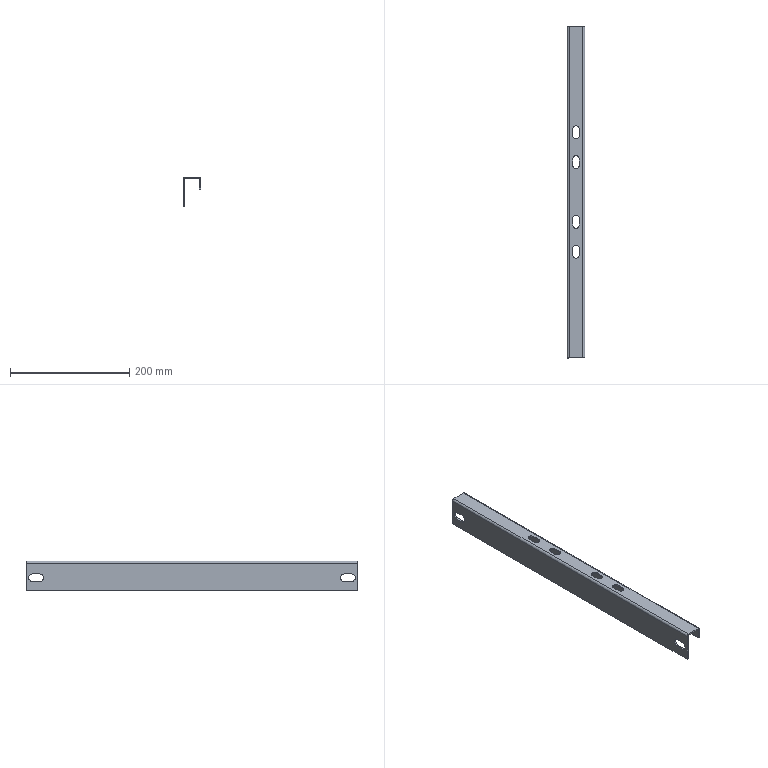Part | SolidWorks | features ICE 2, FlatPattern 1, SMBaseFlange 1, SheetMetal 1 | 1 solid | 46 faces | box 30 x 557 x 50 mm | volume 125994 mm3 | plane 30 | cylinder 16 | commonest cylinder face diameters 11 x8 13 x4 2 x2 7 x2
STEP:
#1=CARTESIAN_POINT('',(0.,278.5,-3.5));
#2=VERTEX_POINT('',#1);
#3=CARTESIAN_POINT('',(2.5,278.5,-3.5));
#4=VERTEX_POINT('',#3);
#5=CARTESIAN_POINT('',(0.,278.5,-3.5));
#6=DIRECTION('',(1.,0.,0.));
#7=VECTOR('',#6,1000.);
#8=LINE('',#5,#7);
#9=EDGE_CURVE('',#2,#4,#8,.T.);
#10=ORIENTED_EDGE('',*,*,#9,.F.);
#11=CARTESIAN_POINT('',(3.5,278.5,0.));
#12=VERTEX_POINT('',#11);
#13=CARTESIAN_POINT('',(3.5,278.5,-3.5));
#14=DIRECTION('',(0.,1.,0.));
#15=DIRECTION('',(0.,0.,-1.));
#16=AXIS2_PLACEMENT_3D('',#13,#14,#15);
#17=CIRCLE('',#16,3.5);
#18=EDGE_CURVE('',#2,#12,#17,.T.);
#19=ORIENTED_EDGE('',*,*,#18,.T.);
#20=CARTESIAN_POINT('',(3.5,278.5,-2.5));
#21=VERTEX_POINT('',#20);
#22=CARTESIAN_POINT('',(3.5,278.5,-2.5));
#23=DIRECTION('',(0.,0.,1.));
#24=VECTOR('',#23,1000.);
#25=LINE('',#22,#24);
#26=EDGE_CURVE('',#21,#12,#25,.T.);
#27=ORIENTED_EDGE('',*,*,#26,.F.);
#28=CARTESIAN_POINT('',(3.5,278.5,-3.5));
#29=DIRECTION('',(0.,1.,0.));
#30=DIRECTION('',(1.,0.,0.));
#31=AXIS2_PLACEMENT_3D('',#28,#29,#30);
#32=CIRCLE('',#31,1.);
#33=EDGE_CURVE('',#4,#21,#32,.T.);
#34=ORIENTED_EDGE('',*,*,#33,.F.);
#35=EDGE_LOOP('',(#10,#19,#27,#34));
#36=FACE_OUTER_BOUND('',#35,.T.);
#37=CARTESIAN_POINT('',(0.,278.5,-3.5));
#38=DIRECTION('',(0.,1.,0.));
#39=DIRECTION('',(0.,0.,1.));
#40=AXIS2_PLACEMENT_3D('',#37,#38,#39);
#41=PLANE('',#40);
#42=ADVANCED_FACE('',(#36),#41,.T.);
#43=CARTESIAN_POINT('',(0.,278.5,-50.));
#44=VERTEX_POINT('',#43);
#45=CARTESIAN_POINT('',(0.,278.5,0.));
#46=DIRECTION('',(0.,0.,1.));
#47=VECTOR('',#46,1000.);
#48=LINE('',#45,#47);
#49=EDGE_CURVE('',#44,#2,#48,.T.);
#50=ORIENTED_EDGE('',*,*,#49,.T.);
#51=ORIENTED_EDGE('',*,*,#9,.T.);
#52=CARTESIAN_POINT('',(2.5,278.5,-50.));
#53=VERTEX_POINT('',#52);
#54=CARTESIAN_POINT('',(2.5,278.5,0.));
#55=DIRECTION('',(0.,0.,1.));
#56=VECTOR('',#55,1000.);
#57=LINE('',#54,#56);
#58=EDGE_CURVE('',#53,#4,#57,.T.);
#59=ORIENTED_EDGE('',*,*,#58,.F.);
#60=CARTESIAN_POINT('',(0.,278.5,-50.));
#61=DIRECTION('',(1.,0.,0.));
#62=VECTOR('',#61,1000.);
#63=LINE('',#60,#62);
#64=EDGE_CURVE('',#44,#53,#63,.T.);
#65=ORIENTED_EDGE('',*,*,#64,.F.);
#66=EDGE_LOOP('',(#50,#51,#59,#65));
#67=FACE_OUTER_BOUND('',#66,.T.);
#68=CARTESIAN_POINT('',(3.5,278.5,-2.5));
#69=DIRECTION('',(0.,1.,0.));
#70=DIRECTION('',(0.,0.,1.));
#71=AXIS2_PLACEMENT_3D('',#68,#69,#70);
#72=PLANE('',#71);
#73=ADVANCED_FACE('',(#67),#72,.T.);
#74=CARTESIAN_POINT('',(3.5,-278.5,0.));
#75=VERTEX_POINT('',#74);
#76=CARTESIAN_POINT('',(3.5,-278.5,-2.5));
#77=VERTEX_POINT('',#76);
#78=CARTESIAN_POINT('',(3.5,-278.5,0.));
#79=DIRECTION('',(0.,0.,-1.));
#80=VECTOR('',#79,1000.);
#81=LINE('',#78,#80);
#82=EDGE_CURVE('',#75,#77,#81,.T.);
#83=ORIENTED_EDGE('',*,*,#82,.F.);
#84=CARTESIAN_POINT('',(0.,-278.5,-3.5));
#85=VERTEX_POINT('',#84);
#86=CARTESIAN_POINT('',(3.5,-278.5,-3.5));
#87=DIRECTION('',(0.,1.,0.));
#88=DIRECTION('',(0.,0.,-1.));
#89=AXIS2_PLACEMENT_3D('',#86,#87,#88);
#90=CIRCLE('',#89,3.5);
#91=EDGE_CURVE('',#85,#75,#90,.T.);
#92=ORIENTED_EDGE('',*,*,#91,.F.);
#93=CARTESIAN_POINT('',(2.5,-278.5,-3.5));
#94=VERTEX_POINT('',#93);
#95=CARTESIAN_POINT('',(2.5,-278.5,-3.5));
#96=DIRECTION('',(-1.,0.,0.));
#97=VECTOR('',#96,1000.);
#98=LINE('',#95,#97);
#99=EDGE_CURVE('',#94,#85,#98,.T.);
#100=ORIENTED_EDGE('',*,*,#99,.F.);
#101=CARTESIAN_POINT('',(3.5,-278.5,-3.5));
#102=DIRECTION('',(0.,1.,0.));
#103=DIRECTION('',(1.,0.,0.));
#104=AXIS2_PLACEMENT_3D('',#101,#102,#103);
#105=CIRCLE('',#104,1.);
#106=EDGE_CURVE('',#94,#77,#105,.T.);
#107=ORIENTED_EDGE('',*,*,#106,.T.);
#108=EDGE_LOOP('',(#83,#92,#100,#107));
#109=FACE_OUTER_BOUND('',#108,.T.);
#110=CARTESIAN_POINT('',(3.5,-278.5,0.));
#111=DIRECTION('',(0.,-1.,0.));
#112=DIRECTION('',(0.,0.,-1.));
#113=AXIS2_PLACEMENT_3D('',#110,#111,#112);
#114=PLANE('',#113);
#115=ADVANCED_FACE('',(#109),#114,.T.);
#116=CARTESIAN_POINT('',(26.5,-278.5,0.));
#117=VERTEX_POINT('',#116);
#118=CARTESIAN_POINT('',(0.,-278.5,0.));
#119=DIRECTION('',(1.,0.,0.));
#120=VECTOR('',#119,1000.);
#121=LINE('',#118,#120);
#122=EDGE_CURVE('',#75,#117,#121,.T.);
#123=ORIENTED_EDGE('',*,*,#122,.F.);
#124=ORIENTED_EDGE('',*,*,#82,.T.);
#125=CARTESIAN_POINT('',(26.5,-278.5,-2.5));
#126=VERTEX_POINT('',#125);
#127=CARTESIAN_POINT('',(0.,-278.5,-2.5));
#128=DIRECTION('',(1.,0.,0.));
#129=VECTOR('',#128,1000.);
#130=LINE('',#127,#129);
#131=EDGE_CURVE('',#77,#126,#130,.T.);
#132=ORIENTED_EDGE('',*,*,#131,.T.);
#133=CARTESIAN_POINT('',(26.5,-278.5,-2.5));
#134=DIRECTION('',(0.,0.,1.));
#135=VECTOR('',#134,1000.);
#136=LINE('',#133,#135);
#137=EDGE_CURVE('',#126,#117,#136,.T.);
#138=ORIENTED_EDGE('',*,*,#137,.T.);
#139=EDGE_LOOP('',(#123,#124,#132,#138));
#140=FACE_OUTER_BOUND('',#139,.T.);
#141=CARTESIAN_POINT('',(2.5,-278.5,-3.5));
#142=DIRECTION('',(0.,-1.,0.));
#143=DIRECTION('',(0.,0.,-1.));
#144=AXIS2_PLACEMENT_3D('',#141,#142,#143);
#145=PLANE('',#144);
#146=ADVANCED_FACE('',(#140),#145,.T.);
#147=CARTESIAN_POINT('',(26.5,278.5,0.));
#148=VERTEX_POINT('',#147);
#149=CARTESIAN_POINT('',(26.5,278.5,-2.5));
#150=VERTEX_POINT('',#149);
#151=CARTESIAN_POINT('',(26.5,278.5,0.));
#152=DIRECTION('',(0.,0.,-1.));
#153=VECTOR('',#152,1000.);
#154=LINE('',#151,#153);
#155=EDGE_CURVE('',#148,#150,#154,.T.);
#156=ORIENTED_EDGE('',*,*,#155,.F.);
#157=CARTESIAN_POINT('',(30.,278.5,-3.5));
#158=VERTEX_POINT('',#157);
#159=CARTESIAN_POINT('',(26.5,278.5,-3.5));
#160=DIRECTION('',(0.,1.,0.));
#161=DIRECTION('',(0.,0.,-1.));
#162=AXIS2_PLACEMENT_3D('',#159,#160,#161);
#163=CIRCLE('',#162,3.5);
#164=EDGE_CURVE('',#148,#158,#163,.T.);
#165=ORIENTED_EDGE('',*,*,#164,.T.);
#166=CARTESIAN_POINT('',(27.5,278.5,-3.5));
#167=VERTEX_POINT('',#166);
#168=CARTESIAN_POINT('',(27.5,278.5,-3.5));
#169=DIRECTION('',(1.,0.,0.));
#170=VECTOR('',#169,1000.);
#171=LINE('',#168,#170);
#172=EDGE_CURVE('',#167,#158,#171,.T.);
#173=ORIENTED_EDGE('',*,*,#172,.F.);
#174=CARTESIAN_POINT('',(26.5,278.5,-3.5));
#175=DIRECTION('',(0.,1.,0.));
#176=DIRECTION('',(1.,0.,0.));
#177=AXIS2_PLACEMENT_3D('',#174,#175,#176);
#178=CIRCLE('',#177,1.);
#179=EDGE_CURVE('',#150,#167,#178,.T.);
#180=ORIENTED_EDGE('',*,*,#179,.F.);
#181=EDGE_LOOP('',(#156,#165,#173,#180));
#182=FACE_OUTER_BOUND('',#181,.T.);
#183=CARTESIAN_POINT('',(26.5,278.5,0.));
#184=DIRECTION('',(0.,1.,0.));
#185=DIRECTION('',(0.,0.,1.));
#186=AXIS2_PLACEMENT_3D('',#183,#184,#185);
#187=PLANE('',#186);
#188=ADVANCED_FACE('',(#182),#187,.T.);
#189=CARTESIAN_POINT('',(0.,278.5,0.));
#190=DIRECTION('',(1.,0.,0.));
#191=VECTOR('',#190,1000.);
#192=LINE('',#189,#191);
#193=EDGE_CURVE('',#12,#148,#192,.T.);
#194=ORIENTED_EDGE('',*,*,#193,.T.);
#195=ORIENTED_EDGE('',*,*,#155,.T.);
#196=CARTESIAN_POINT('',(0.,278.5,-2.5));
#197=DIRECTION('',(1.,0.,0.));
#198=VECTOR('',#197,1000.);
#199=LINE('',#196,#198);
#200=EDGE_CURVE('',#21,#150,#199,.T.);
#201=ORIENTED_EDGE('',*,*,#200,.F.);
#202=ORIENTED_EDGE('',*,*,#26,.T.);
#203=EDGE_LOOP('',(#194,#195,#201,#202));
#204=FACE_OUTER_BOUND('',#203,.T.);
#205=CARTESIAN_POINT('',(27.5,278.5,-3.5));
#206=DIRECTION('',(0.,1.,0.));
#207=DIRECTION('',(0.,0.,1.));
#208=AXIS2_PLACEMENT_3D('',#205,#206,#207);
#209=PLANE('',#208);
#210=ADVANCED_FACE('',(#204),#209,.T.);
#211=CARTESIAN_POINT('',(30.,-278.5,-3.5));
#212=VERTEX_POINT('',#211);
#213=CARTESIAN_POINT('',(27.5,-278.5,-3.5));
#214=VERTEX_POINT('',#213);
#215=CARTESIAN_POINT('',(30.,-278.5,-3.5));
#216=DIRECTION('',(-1.,0.,0.));
#217=VECTOR('',#216,1000.);
#218=LINE('',#215,#217);
#219=EDGE_CURVE('',#212,#214,#218,.T.);
#220=ORIENTED_EDGE('',*,*,#219,.F.);
#221=CARTESIAN_POINT('',(26.5,-278.5,-3.5));
#222=DIRECTION('',(0.,1.,0.));
#223=DIRECTION('',(0.,0.,-1.));
#224=AXIS2_PLACEMENT_3D('',#221,#222,#223);
#225=CIRCLE('',#224,3.5);
#226=EDGE_CURVE('',#117,#212,#225,.T.);
#227=ORIENTED_EDGE('',*,*,#226,.F.);
#228=ORIENTED_EDGE('',*,*,#137,.F.);
#229=CARTESIAN_POINT('',(26.5,-278.5,-3.5));
#230=DIRECTION('',(0.,1.,0.));
#231=DIRECTION('',(1.,0.,0.));
#232=AXIS2_PLACEMENT_3D('',#229,#230,#231);
#233=CIRCLE('',#232,1.);
#234=EDGE_CURVE('',#126,#214,#233,.T.);
#235=ORIENTED_EDGE('',*,*,#234,.T.);
#236=EDGE_LOOP('',(#220,#227,#228,#235));
#237=FACE_OUTER_BOUND('',#236,.T.);
#238=CARTESIAN_POINT('',(30.,-278.5,-3.5));
#239=DIRECTION('',(0.,-1.,0.));
#240=DIRECTION('',(0.,0.,-1.));
#241=AXIS2_PLACEMENT_3D('',#238,#239,#240);
#242=PLANE('',#241);
#243=ADVANCED_FACE('',(#237),#242,.T.);
#244=CARTESIAN_POINT('',(30.,-278.5,-20.));
#245=VERTEX_POINT('',#244);
#246=CARTESIAN_POINT('',(30.,-278.5,0.));
#247=DIRECTION('',(0.,0.,-1.));
#248=VECTOR('',#247,1000.);
#249=LINE('',#246,#248);
#250=EDGE_CURVE('',#212,#245,#249,.T.);
#251=ORIENTED_EDGE('',*,*,#250,.F.);
#252=ORIENTED_EDGE('',*,*,#219,.T.);
#253=CARTESIAN_POINT('',(27.5,-278.5,-20.));
#254=VERTEX_POINT('',#253);
#255=CARTESIAN_POINT('',(27.5,-278.5,0.));
#256=DIRECTION('',(0.,0.,-1.));
#257=VECTOR('',#256,1000.);
#258=LINE('',#255,#257);
#259=EDGE_CURVE('',#214,#254,#258,.T.);
#260=ORIENTED_EDGE('',*,*,#259,.T.);
#261=CARTESIAN_POINT('',(27.5,-278.5,-20.));
#262=DIRECTION('',(1.,0.,0.));
#263=VECTOR('',#262,1000.);
#264=LINE('',#261,#263);
#265=EDGE_CURVE('',#254,#245,#264,.T.);
#266=ORIENTED_EDGE('',*,*,#265,.T.);
#267=EDGE_LOOP('',(#251,#252,#260,#266));
#268=FACE_OUTER_BOUND('',#267,.T.);
#269=CARTESIAN_POINT('',(26.5,-278.5,-2.5));
#270=DIRECTION('',(0.,-1.,0.));
#271=DIRECTION('',(0.,0.,-1.));
#272=AXIS2_PLACEMENT_3D('',#269,#270,#271);
#273=PLANE('',#272);
#274=ADVANCED_FACE('',(#268),#273,.T.);
#275=ORIENTED_EDGE('',*,*,#250,.T.);
#276=CARTESIAN_POINT('',(30.,278.5,-20.));
#277=VERTEX_POINT('',#276);
#278=CARTESIAN_POINT('',(30.,278.5,-20.));
#279=DIRECTION('',(0.,-1.,0.));
#280=VECTOR('',#279,1000.);
#281=LINE('',#278,#280);
#282=EDGE_CURVE('',#277,#245,#281,.T.);
#283=ORIENTED_EDGE('',*,*,#282,.F.);
#284=CARTESIAN_POINT('',(30.,278.5,0.));
#285=DIRECTION('',(0.,0.,-1.));
#286=VECTOR('',#285,1000.);
#287=LINE('',#284,#286);
#288=EDGE_CURVE('',#158,#277,#287,.T.);
#289=ORIENTED_EDGE('',*,*,#288,.F.);
#290=CARTESIAN_POINT('',(30.,278.5,-3.5));
#291=DIRECTION('',(0.,-1.,0.));
#292=VECTOR('',#291,1000.);
#293=LINE('',#290,#292);
#294=EDGE_CURVE('',#158,#212,#293,.T.);
#295=ORIENTED_EDGE('',*,*,#294,.T.);
#296=EDGE_LOOP('',(#275,#283,#289,#295));
#297=FACE_OUTER_BOUND('',#296,.T.);
#298=CARTESIAN_POINT('',(30.,278.5,0.));
#299=DIRECTION('',(-1.,0.,0.));
#300=DIRECTION('',(0.,0.,1.));
#301=AXIS2_PLACEMENT_3D('',#298,#299,#300);
#302=PLANE('',#301);
#303=ADVANCED_FACE('',(#297),#302,.F.);
#304=ORIENTED_EDGE('',*,*,#265,.F.);
#305=CARTESIAN_POINT('',(27.5,278.5,-20.));
#306=VERTEX_POINT('',#305);
#307=CARTESIAN_POINT('',(27.5,278.5,-20.));
#308=DIRECTION('',(0.,-1.,0.));
#309=VECTOR('',#308,1000.);
#310=LINE('',#307,#309);
#311=EDGE_CURVE('',#306,#254,#310,.T.);
#312=ORIENTED_EDGE('',*,*,#311,.F.);
#313=CARTESIAN_POINT('',(27.5,278.5,-20.));
#314=DIRECTION('',(1.,0.,0.));
#315=VECTOR('',#314,1000.);
#316=LINE('',#313,#315);
#317=EDGE_CURVE('',#306,#277,#316,.T.);
#318=ORIENTED_EDGE('',*,*,#317,.T.);
#319=ORIENTED_EDGE('',*,*,#282,.T.);
#320=EDGE_LOOP('',(#304,#312,#318,#319));
#321=FACE_OUTER_BOUND('',#320,.T.);
#322=CARTESIAN_POINT('',(27.5,278.5,-20.));
#323=DIRECTION('',(0.,0.,-1.));
#324=DIRECTION('',(-1.,0.,0.));
#325=AXIS2_PLACEMENT_3D('',#322,#323,#324);
#326=PLANE('',#325);
#327=ADVANCED_FACE('',(#321),#326,.T.);
#328=ORIENTED_EDGE('',*,*,#259,.F.);
#329=CARTESIAN_POINT('',(27.5,278.5,-3.5));
#330=DIRECTION('',(0.,-1.,0.));
#331=VECTOR('',#330,1000.);
#332=LINE('',#329,#331);
#333=EDGE_CURVE('',#167,#214,#332,.T.);
#334=ORIENTED_EDGE('',*,*,#333,.F.);
#335=CARTESIAN_POINT('',(27.5,278.5,0.));
#336=DIRECTION('',(0.,0.,-1.));
#337=VECTOR('',#336,1000.);
#338=LINE('',#335,#337);
#339=EDGE_CURVE('',#167,#306,#338,.T.);
#340=ORIENTED_EDGE('',*,*,#339,.T.);
#341=ORIENTED_EDGE('',*,*,#311,.T.);
#342=EDGE_LOOP('',(#328,#334,#340,#341));
#343=FACE_OUTER_BOUND('',#342,.T.);
#344=CARTESIAN_POINT('',(27.5,278.5,0.));
#345=DIRECTION('',(-1.,0.,0.));
#346=DIRECTION('',(0.,0.,1.));
#347=AXIS2_PLACEMENT_3D('',#344,#345,#346);
#348=PLANE('',#347);
#349=ADVANCED_FACE('',(#343),#348,.T.);
#350=ORIENTED_EDGE('',*,*,#234,.F.);
#351=CARTESIAN_POINT('',(26.5,278.5,-2.5));
#352=DIRECTION('',(0.,-1.,0.));
#353=VECTOR('',#352,1000.);
#354=LINE('',#351,#353);
#355=EDGE_CURVE('',#150,#126,#354,.T.);
#356=ORIENTED_EDGE('',*,*,#355,.F.);
#357=ORIENTED_EDGE('',*,*,#179,.T.);
#358=ORIENTED_EDGE('',*,*,#333,.T.);
#359=EDGE_LOOP('',(#350,#356,#357,#358));
#360=FACE_OUTER_BOUND('',#359,.T.);
#361=CARTESIAN_POINT('',(26.5,278.5,-3.5));
#362=DIRECTION('',(0.,-1.,0.));
#363=DIRECTION('',(0.,0.,-1.));
#364=AXIS2_PLACEMENT_3D('',#361,#362,#363);
#365=CYLINDRICAL_SURFACE('',#364,1.);
#366=ADVANCED_FACE('',(#360),#365,.F.);
#367=CARTESIAN_POINT('',(20.5,-105.5,-2.5));
#368=VERTEX_POINT('',#367);
#369=CARTESIAN_POINT('',(9.5,-105.5,-2.5));
#370=VERTEX_POINT('',#369);
#371=CARTESIAN_POINT('',(15.,-105.5,-2.5));
#372=DIRECTION('',(0.,0.,-1.));
#373=DIRECTION('',(-1.,0.,0.));
#374=AXIS2_PLACEMENT_3D('',#371,#372,#373);
#375=CIRCLE('',#374,5.5);
#376=EDGE_CURVE('',#368,#370,#375,.T.);
#377=ORIENTED_EDGE('',*,*,#376,.F.);
#378=CARTESIAN_POINT('',(20.5,-94.5,-2.5));
#379=VERTEX_POINT('',#378);
#380=CARTESIAN_POINT('',(20.5,-105.5,-2.5));
#381=DIRECTION('',(0.,-1.,0.));
#382=VECTOR('',#381,1000.);
#383=LINE('',#380,#382);
#384=EDGE_CURVE('',#379,#368,#383,.T.);
#385=ORIENTED_EDGE('',*,*,#384,.F.);
#386=CARTESIAN_POINT('',(9.5,-94.5,-2.5));
#387=VERTEX_POINT('',#386);
#388=CARTESIAN_POINT('',(15.,-94.5,-2.5));
#389=DIRECTION('',(0.,0.,-1.));
#390=DIRECTION('',(-1.,0.,0.));
#391=AXIS2_PLACEMENT_3D('',#388,#389,#390);
#392=CIRCLE('',#391,5.5);
#393=EDGE_CURVE('',#387,#379,#392,.T.);
#394=ORIENTED_EDGE('',*,*,#393,.F.);
#395=CARTESIAN_POINT('',(9.5,-105.5,-2.5));
#396=DIRECTION('',(0.,1.,0.));
#397=VECTOR('',#396,1000.);
#398=LINE('',#395,#397);
#399=EDGE_CURVE('',#370,#387,#398,.T.);
#400=ORIENTED_EDGE('',*,*,#399,.F.);
#401=EDGE_LOOP('',(#377,#385,#394,#400));
#402=FACE_BOUND('',#401,.T.);
#403=CARTESIAN_POINT('',(9.5,105.5,-2.5));
#404=VERTEX_POINT('',#403);
#405=CARTESIAN_POINT('',(20.5,105.5,-2.5));
#406=VERTEX_POINT('',#405);
#407=CARTESIAN_POINT('',(15.,105.5,-2.5));
#408=DIRECTION('',(0.,0.,-1.));
#409=DIRECTION('',(1.,0.,0.));
#410=AXIS2_PLACEMENT_3D('',#407,#408,#409);
#411=CIRCLE('',#410,5.5);
#412=EDGE_CURVE('',#404,#406,#411,.T.);
#413=ORIENTED_EDGE('',*,*,#412,.F.);
#414=CARTESIAN_POINT('',(9.5,94.5,-2.5));
#415=VERTEX_POINT('',#414);
#416=CARTESIAN_POINT('',(9.5,105.5,-2.5));
#417=DIRECTION('',(0.,1.,0.));
#418=VECTOR('',#417,1000.);
#419=LINE('',#416,#418);
#420=EDGE_CURVE('',#415,#404,#419,.T.);
#421=ORIENTED_EDGE('',*,*,#420,.F.);
#422=CARTESIAN_POINT('',(20.5,94.5,-2.5));
#423=VERTEX_POINT('',#422);
#424=CARTESIAN_POINT('',(15.,94.5,-2.5));
#425=DIRECTION('',(0.,0.,-1.));
#426=DIRECTION('',(1.,0.,0.));
#427=AXIS2_PLACEMENT_3D('',#424,#425,#426);
#428=CIRCLE('',#427,5.5);
#429=EDGE_CURVE('',#423,#415,#428,.T.);
#430=ORIENTED_EDGE('',*,*,#429,.F.);
#431=CARTESIAN_POINT('',(20.5,105.5,-2.5));
#432=DIRECTION('',(0.,-1.,0.));
#433=VECTOR('',#432,1000.);
#434=LINE('',#431,#433);
#435=EDGE_CURVE('',#406,#423,#434,.T.);
#436=ORIENTED_EDGE('',*,*,#435,.F.);
#437=EDGE_LOOP('',(#413,#421,#430,#436));
#438=FACE_BOUND('',#437,.T.);
#439=CARTESIAN_POINT('',(9.5,55.5,-2.5));
#440=VERTEX_POINT('',#439);
#441=CARTESIAN_POINT('',(20.5,55.5,-2.5));
#442=VERTEX_POINT('',#441);
#443=CARTESIAN_POINT('',(15.,55.5,-2.5));
#444=DIRECTION('',(0.,0.,-1.));
#445=DIRECTION('',(1.,0.,0.));
#446=AXIS2_PLACEMENT_3D('',#443,#444,#445);
#447=CIRCLE('',#446,5.5);
#448=EDGE_CURVE('',#440,#442,#447,.T.);
#449=ORIENTED_EDGE('',*,*,#448,.F.);
#450=CARTESIAN_POINT('',(9.5,44.5,-2.5));
#451=VERTEX_POINT('',#450);
#452=CARTESIAN_POINT('',(9.5,55.5,-2.5));
#453=DIRECTION('',(0.,1.,0.));
#454=VECTOR('',#453,1000.);
#455=LINE('',#452,#454);
#456=EDGE_CURVE('',#451,#440,#455,.T.);
#457=ORIENTED_EDGE('',*,*,#456,.F.);
#458=CARTESIAN_POINT('',(20.5,44.5,-2.5));
#459=VERTEX_POINT('',#458);
#460=CARTESIAN_POINT('',(15.,44.5,-2.5));
#461=DIRECTION('',(0.,0.,-1.));
#462=DIRECTION('',(1.,0.,0.));
#463=AXIS2_PLACEMENT_3D('',#460,#461,#462);
#464=CIRCLE('',#463,5.5);
#465=EDGE_CURVE('',#459,#451,#464,.T.);
#466=ORIENTED_EDGE('',*,*,#465,.F.);
#467=CARTESIAN_POINT('',(20.5,55.5,-2.5));
#468=DIRECTION('',(0.,-1.,0.));
#469=VECTOR('',#468,1000.);
#470=LINE('',#467,#469);
#471=EDGE_CURVE('',#442,#459,#470,.T.);
#472=ORIENTED_EDGE('',*,*,#471,.F.);
#473=EDGE_LOOP('',(#449,#457,#466,#472));
#474=FACE_BOUND('',#473,.T.);
#475=CARTESIAN_POINT('',(20.5,-55.5,-2.5));
#476=VERTEX_POINT('',#475);
#477=CARTESIAN_POINT('',(9.5,-55.5,-2.5));
#478=VERTEX_POINT('',#477);
#479=CARTESIAN_POINT('',(15.,-55.5,-2.5));
#480=DIRECTION('',(0.,0.,-1.));
#481=DIRECTION('',(-1.,0.,0.));
#482=AXIS2_PLACEMENT_3D('',#479,#480,#481);
#483=CIRCLE('',#482,5.5);
#484=EDGE_CURVE('',#476,#478,#483,.T.);
#485=ORIENTED_EDGE('',*,*,#484,.F.);
#486=CARTESIAN_POINT('',(20.5,-44.5,-2.5));
#487=VERTEX_POINT('',#486);
#488=CARTESIAN_POINT('',(20.5,-55.5,-2.5));
#489=DIRECTION('',(0.,-1.,0.));
#490=VECTOR('',#489,1000.);
#491=LINE('',#488,#490);
#492=EDGE_CURVE('',#487,#476,#491,.T.);
#493=ORIENTED_EDGE('',*,*,#492,.F.);
#494=CARTESIAN_POINT('',(9.5,-44.5,-2.5));
#495=VERTEX_POINT('',#494);
#496=CARTESIAN_POINT('',(15.,-44.5,-2.5));
#497=DIRECTION('',(0.,0.,-1.));
#498=DIRECTION('',(-1.,0.,0.));
#499=AXIS2_PLACEMENT_3D('',#496,#497,#498);
#500=CIRCLE('',#499,5.5);
#501=EDGE_CURVE('',#495,#487,#500,.T.);
#502=ORIENTED_EDGE('',*,*,#501,.F.);
#503=CARTESIAN_POINT('',(9.5,-55.5,-2.5));
#504=DIRECTION('',(0.,1.,0.));
#505=VECTOR('',#504,1000.);
#506=LINE('',#503,#505);
#507=EDGE_CURVE('',#478,#495,#506,.T.);
#508=ORIENTED_EDGE('',*,*,#507,.F.);
#509=EDGE_LOOP('',(#485,#493,#502,#508));
#510=FACE_BOUND('',#509,.T.);
#511=ORIENTED_EDGE('',*,*,#131,.F.);
#512=CARTESIAN_POINT('',(3.5,278.5,-2.5));
#513=DIRECTION('',(0.,-1.,0.));
#514=VECTOR('',#513,1000.);
#515=LINE('',#512,#514);
#516=EDGE_CURVE('',#21,#77,#515,.T.);
#517=ORIENTED_EDGE('',*,*,#516,.F.);
#518=ORIENTED_EDGE('',*,*,#200,.T.);
#519=ORIENTED_EDGE('',*,*,#355,.T.);
#520=EDGE_LOOP('',(#511,#517,#518,#519));
#521=FACE_OUTER_BOUND('',#520,.T.);
#522=CARTESIAN_POINT('',(0.,278.5,-2.5));
#523=DIRECTION('',(0.,0.,-1.));
#524=DIRECTION('',(-1.,0.,0.));
#525=AXIS2_PLACEMENT_3D('',#522,#523,#524);
#526=PLANE('',#525);
#527=ADVANCED_FACE('',(#402,#438,#474,#510,#521),#526,.T.);
#528=ORIENTED_EDGE('',*,*,#106,.F.);
#529=CARTESIAN_POINT('',(2.5,278.5,-3.5));
#530=DIRECTION('',(0.,-1.,0.));
#531=VECTOR('',#530,1000.);
#532=LINE('',#529,#531);
#533=EDGE_CURVE('',#4,#94,#532,.T.);
#534=ORIENTED_EDGE('',*,*,#533,.F.);
#535=ORIENTED_EDGE('',*,*,#33,.T.);
#536=ORIENTED_EDGE('',*,*,#516,.T.);
#537=EDGE_LOOP('',(#528,#534,#535,#536));
#538=FACE_OUTER_BOUND('',#537,.T.);
#539=CARTESIAN_POINT('',(3.5,278.5,-3.5));
#540=DIRECTION('',(0.,-1.,0.));
#541=DIRECTION('',(0.,0.,-1.));
#542=AXIS2_PLACEMENT_3D('',#539,#540,#541);
#543=CYLINDRICAL_SURFACE('',#542,1.);
#544=ADVANCED_FACE('',(#538),#543,.F.);
#545=CARTESIAN_POINT('',(2.5,-267.5,-21.5));
#546=VERTEX_POINT('',#545);
#547=CARTESIAN_POINT('',(2.5,-267.5,-34.5));
#548=VERTEX_POINT('',#547);
#549=CARTESIAN_POINT('',(2.5,-267.5,-28.));
#550=DIRECTION('',(1.,0.,0.));
#551=DIRECTION('',(0.,0.,-1.));
#552=AXIS2_PLACEMENT_3D('',#549,#550,#551);
#553=CIRCLE('',#552,6.5);
#554=EDGE_CURVE('',#546,#548,#553,.T.);
#555=ORIENTED_EDGE('',*,*,#554,.F.);
#556=CARTESIAN_POINT('',(2.5,-255.5,-21.5));
#557=VERTEX_POINT('',#556);
#558=CARTESIAN_POINT('',(2.5,278.5,-21.5));
#559=DIRECTION('',(0.,-1.,0.));
#560=VECTOR('',#559,1000.);
#561=LINE('',#558,#560);
#562=EDGE_CURVE('',#557,#546,#561,.T.);
#563=ORIENTED_EDGE('',*,*,#562,.F.);
#564=CARTESIAN_POINT('',(2.5,-255.5,-34.5));
#565=VERTEX_POINT('',#564);
#566=CARTESIAN_POINT('',(2.5,-255.5,-28.));
#567=DIRECTION('',(1.,0.,0.));
#568=DIRECTION('',(0.,0.,-1.));
#569=AXIS2_PLACEMENT_3D('',#566,#567,#568);
#570=CIRCLE('',#569,6.5);
#571=EDGE_CURVE('',#565,#557,#570,.T.);
#572=ORIENTED_EDGE('',*,*,#571,.F.);
#573=CARTESIAN_POINT('',(2.5,278.5,-34.5));
#574=DIRECTION('',(0.,1.,0.));
#575=VECTOR('',#574,1000.);
#576=LINE('',#573,#575);
#577=EDGE_CURVE('',#548,#565,#576,.T.);
#578=ORIENTED_EDGE('',*,*,#577,.F.);
#579=EDGE_LOOP('',(#555,#563,#572,#578));
#580=FACE_BOUND('',#579,.T.);
#581=CARTESIAN_POINT('',(2.5,267.5,-34.5));
#582=VERTEX_POINT('',#581);
#583=CARTESIAN_POINT('',(2.5,267.5,-21.5));
#584=VERTEX_POINT('',#583);
#585=CARTESIAN_POINT('',(2.5,267.5,-28.));
#586=DIRECTION('',(1.,0.,0.));
#587=DIRECTION('',(0.,0.,-1.));
#588=AXIS2_PLACEMENT_3D('',#585,#586,#587);
#589=CIRCLE('',#588,6.5);
#590=EDGE_CURVE('',#582,#584,#589,.T.);
#591=ORIENTED_EDGE('',*,*,#590,.F.);
#592=CARTESIAN_POINT('',(2.5,255.5,-34.5));
#593=VERTEX_POINT('',#592);
#594=CARTESIAN_POINT('',(2.5,278.5,-34.5));
#595=DIRECTION('',(0.,1.,0.));
#596=VECTOR('',#595,1000.);
#597=LINE('',#594,#596);
#598=EDGE_CURVE('',#593,#582,#597,.T.);
#599=ORIENTED_EDGE('',*,*,#598,.F.);
#600=CARTESIAN_POINT('',(2.5,255.5,-21.5));
#601=VERTEX_POINT('',#600);
#602=CARTESIAN_POINT('',(2.5,255.5,-28.));
#603=DIRECTION('',(1.,0.,0.));
#604=DIRECTION('',(0.,0.,-1.));
#605=AXIS2_PLACEMENT_3D('',#602,#603,#604);
#606=CIRCLE('',#605,6.5);
#607=EDGE_CURVE('',#601,#593,#606,.T.);
#608=ORIENTED_EDGE('',*,*,#607,.F.);
#609=CARTESIAN_POINT('',(2.5,278.5,-21.5));
#610=DIRECTION('',(0.,-1.,0.));
#611=VECTOR('',#610,1000.);
#612=LINE('',#609,#611);
#613=EDGE_CURVE('',#584,#601,#612,.T.);
#614=ORIENTED_EDGE('',*,*,#613,.F.);
#615=EDGE_LOOP('',(#591,#599,#608,#614));
#616=FACE_BOUND('',#615,.T.);
#617=CARTESIAN_POINT('',(2.5,-278.5,-50.));
#618=VERTEX_POINT('',#617);
#619=CARTESIAN_POINT('',(2.5,-278.5,0.));
#620=DIRECTION('',(0.,0.,1.));
#621=VECTOR('',#620,1000.);
#622=LINE('',#619,#621);
#623=EDGE_CURVE('',#618,#94,#622,.T.);
#624=ORIENTED_EDGE('',*,*,#623,.F.);
#625=CARTESIAN_POINT('',(2.5,278.5,-50.));
#626=DIRECTION('',(0.,-1.,0.));
#627=VECTOR('',#626,1000.);
#628=LINE('',#625,#627);
#629=EDGE_CURVE('',#53,#618,#628,.T.);
#630=ORIENTED_EDGE('',*,*,#629,.F.);
#631=ORIENTED_EDGE('',*,*,#58,.T.);
#632=ORIENTED_EDGE('',*,*,#533,.T.);
#633=EDGE_LOOP('',(#624,#630,#631,#632));
#634=FACE_OUTER_BOUND('',#633,.T.);
#635=CARTESIAN_POINT('',(2.5,278.5,0.));
#636=DIRECTION('',(1.,0.,0.));
#637=DIRECTION('',(0.,0.,-1.));
#638=AXIS2_PLACEMENT_3D('',#635,#636,#637);
#639=PLANE('',#638);
#640=ADVANCED_FACE('',(#580,#616,#634),#639,.T.);
#641=CARTESIAN_POINT('',(0.,-278.5,-50.));
#642=VERTEX_POINT('',#641);
#643=CARTESIAN_POINT('',(0.,-278.5,-50.));
#644=DIRECTION('',(1.,0.,0.));
#645=VECTOR('',#644,1000.);
#646=LINE('',#643,#645);
#647=EDGE_CURVE('',#642,#618,#646,.T.);
#648=ORIENTED_EDGE('',*,*,#647,.F.);
#649=CARTESIAN_POINT('',(0.,278.5,-50.));
#650=DIRECTION('',(0.,-1.,0.));
#651=VECTOR('',#650,1000.);
#652=LINE('',#649,#651);
#653=EDGE_CURVE('',#44,#642,#652,.T.);
#654=ORIENTED_EDGE('',*,*,#653,.F.);
#655=ORIENTED_EDGE('',*,*,#64,.T.);
#656=ORIENTED_EDGE('',*,*,#629,.T.);
#657=EDGE_LOOP('',(#648,#654,#655,#656));
#658=FACE_OUTER_BOUND('',#657,.T.);
#659=CARTESIAN_POINT('',(0.,278.5,-50.));
#660=DIRECTION('',(0.,0.,-1.));
#661=DIRECTION('',(-1.,0.,0.));
#662=AXIS2_PLACEMENT_3D('',#659,#660,#661);
#663=PLANE('',#662);
#664=ADVANCED_FACE('',(#658),#663,.T.);
#665=CARTESIAN_POINT('',(0.,-267.5,-21.5));
#666=VERTEX_POINT('',#665);
#667=CARTESIAN_POINT('',(0.,-255.5,-21.5));
#668=VERTEX_POINT('',#667);
#669=CARTESIAN_POINT('',(0.,-267.5,-21.5));
#670=DIRECTION('',(0.,1.,0.));
#671=VECTOR('',#670,1000.);
#672=LINE('',#669,#671);
#673=EDGE_CURVE('',#666,#668,#672,.T.);
#674=ORIENTED_EDGE('',*,*,#673,.F.);
#675=CARTESIAN_POINT('',(0.,-267.5,-34.5));
#676=VERTEX_POINT('',#675);
#677=CARTESIAN_POINT('',(0.,-267.5,-28.));
#678=DIRECTION('',(-1.,0.,0.));
#679=DIRECTION('',(0.,0.,1.));
#680=AXIS2_PLACEMENT_3D('',#677,#678,#679);
#681=CIRCLE('',#680,6.5);
#682=EDGE_CURVE('',#676,#666,#681,.T.);
#683=ORIENTED_EDGE('',*,*,#682,.F.);
#684=CARTESIAN_POINT('',(0.,-255.5,-34.5));
#685=VERTEX_POINT('',#684);
#686=CARTESIAN_POINT('',(0.,-267.5,-34.5));
#687=DIRECTION('',(0.,-1.,0.));
#688=VECTOR('',#687,1000.);
#689=LINE('',#686,#688);
#690=EDGE_CURVE('',#685,#676,#689,.T.);
#691=ORIENTED_EDGE('',*,*,#690,.F.);
#692=CARTESIAN_POINT('',(0.,-255.5,-28.));
#693=DIRECTION('',(-1.,0.,0.));
#694=DIRECTION('',(0.,0.,1.));
#695=AXIS2_PLACEMENT_3D('',#692,#693,#694);
#696=CIRCLE('',#695,6.5);
#697=EDGE_CURVE('',#668,#685,#696,.T.);
#698=ORIENTED_EDGE('',*,*,#697,.F.);
#699=EDGE_LOOP('',(#674,#683,#691,#698));
#700=FACE_BOUND('',#699,.T.);
#701=CARTESIAN_POINT('',(0.,267.5,-34.5));
#702=VERTEX_POINT('',#701);
#703=CARTESIAN_POINT('',(0.,255.5,-34.5));
#704=VERTEX_POINT('',#703);
#705=CARTESIAN_POINT('',(0.,267.5,-34.5));
#706=DIRECTION('',(0.,-1.,0.));
#707=VECTOR('',#706,1000.);
#708=LINE('',#705,#707);
#709=EDGE_CURVE('',#702,#704,#708,.T.);
#710=ORIENTED_EDGE('',*,*,#709,.F.);
#711=CARTESIAN_POINT('',(0.,267.5,-21.5));
#712=VERTEX_POINT('',#711);
#713=CARTESIAN_POINT('',(0.,267.5,-28.));
#714=DIRECTION('',(-1.,0.,0.));
#715=DIRECTION('',(0.,0.,-1.));
#716=AXIS2_PLACEMENT_3D('',#713,#714,#715);
#717=CIRCLE('',#716,6.5);
#718=EDGE_CURVE('',#712,#702,#717,.T.);
#719=ORIENTED_EDGE('',*,*,#718,.F.);
#720=CARTESIAN_POINT('',(0.,255.5,-21.5));
#721=VERTEX_POINT('',#720);
#722=CARTESIAN_POINT('',(0.,267.5,-21.5));
#723=DIRECTION('',(0.,1.,0.));
#724=VECTOR('',#723,1000.);
#725=LINE('',#722,#724);
#726=EDGE_CURVE('',#721,#712,#725,.T.);
#727=ORIENTED_EDGE('',*,*,#726,.F.);
#728=CARTESIAN_POINT('',(0.,255.5,-28.));
#729=DIRECTION('',(-1.,0.,0.));
#730=DIRECTION('',(0.,0.,-1.));
#731=AXIS2_PLACEMENT_3D('',#728,#729,#730);
#732=CIRCLE('',#731,6.5);
#733=EDGE_CURVE('',#704,#721,#732,.T.);
#734=ORIENTED_EDGE('',*,*,#733,.F.);
#735=EDGE_LOOP('',(#710,#719,#727,#734));
#736=FACE_BOUND('',#735,.T.);
#737=CARTESIAN_POINT('',(0.,-278.5,0.));
#738=DIRECTION('',(0.,0.,1.));
#739=VECTOR('',#738,1000.);
#740=LINE('',#737,#739);
#741=EDGE_CURVE('',#642,#85,#740,.T.);
#742=ORIENTED_EDGE('',*,*,#741,.T.);
#743=CARTESIAN_POINT('',(0.,278.5,-3.5));
#744=DIRECTION('',(0.,-1.,0.));
#745=VECTOR('',#744,1000.);
#746=LINE('',#743,#745);
#747=EDGE_CURVE('',#2,#85,#746,.T.);
#748=ORIENTED_EDGE('',*,*,#747,.F.);
#749=ORIENTED_EDGE('',*,*,#49,.F.);
#750=ORIENTED_EDGE('',*,*,#653,.T.);
#751=EDGE_LOOP('',(#742,#748,#749,#750));
#752=FACE_OUTER_BOUND('',#751,.T.);
#753=CARTESIAN_POINT('',(0.,278.5,0.));
#754=DIRECTION('',(1.,0.,0.));
#755=DIRECTION('',(0.,0.,-1.));
#756=AXIS2_PLACEMENT_3D('',#753,#754,#755);
#757=PLANE('',#756);
#758=ADVANCED_FACE('',(#700,#736,#752),#757,.F.);
#759=ORIENTED_EDGE('',*,*,#91,.T.);
#760=CARTESIAN_POINT('',(3.5,278.5,0.));
#761=DIRECTION('',(0.,-1.,0.));
#762=VECTOR('',#761,1000.);
#763=LINE('',#760,#762);
#764=EDGE_CURVE('',#12,#75,#763,.T.);
#765=ORIENTED_EDGE('',*,*,#764,.F.);
#766=ORIENTED_EDGE('',*,*,#18,.F.);
#767=ORIENTED_EDGE('',*,*,#747,.T.);
#768=EDGE_LOOP('',(#759,#765,#766,#767));
#769=FACE_OUTER_BOUND('',#768,.T.);
#770=CARTESIAN_POINT('',(3.5,278.5,-3.5));
#771=DIRECTION('',(0.,-1.,0.));
#772=DIRECTION('',(0.,0.,-1.));
#773=AXIS2_PLACEMENT_3D('',#770,#771,#772);
#774=CYLINDRICAL_SURFACE('',#773,3.5);
#775=ADVANCED_FACE('',(#769),#774,.T.);
#776=CARTESIAN_POINT('',(20.5,-94.5,0.));
#777=VERTEX_POINT('',#776);
#778=CARTESIAN_POINT('',(20.5,-105.5,0.));
#779=VERTEX_POINT('',#778);
#780=CARTESIAN_POINT('',(20.5,278.5,0.));
#781=DIRECTION('',(0.,-1.,0.));
#782=VECTOR('',#781,1000.);
#783=LINE('',#780,#782);
#784=EDGE_CURVE('',#777,#779,#783,.T.);
#785=ORIENTED_EDGE('',*,*,#784,.T.);
#786=CARTESIAN_POINT('',(9.5,-105.5,0.));
#787=VERTEX_POINT('',#786);
#788=CARTESIAN_POINT('',(15.,-105.5,0.));
#789=DIRECTION('',(0.,0.,-1.));
#790=DIRECTION('',(-1.,0.,0.));
#791=AXIS2_PLACEMENT_3D('',#788,#789,#790);
#792=CIRCLE('',#791,5.5);
#793=EDGE_CURVE('',#779,#787,#792,.T.);
#794=ORIENTED_EDGE('',*,*,#793,.T.);
#795=CARTESIAN_POINT('',(9.5,-94.5,0.));
#796=VERTEX_POINT('',#795);
#797=CARTESIAN_POINT('',(9.5,278.5,0.));
#798=DIRECTION('',(0.,1.,0.));
#799=VECTOR('',#798,1000.);
#800=LINE('',#797,#799);
#801=EDGE_CURVE('',#787,#796,#800,.T.);
#802=ORIENTED_EDGE('',*,*,#801,.T.);
#803=CARTESIAN_POINT('',(15.,-94.5,0.));
#804=DIRECTION('',(0.,0.,-1.));
#805=DIRECTION('',(-1.,0.,0.));
#806=AXIS2_PLACEMENT_3D('',#803,#804,#805);
#807=CIRCLE('',#806,5.5);
#808=EDGE_CURVE('',#796,#777,#807,.T.);
#809=ORIENTED_EDGE('',*,*,#808,.T.);
#810=EDGE_LOOP('',(#785,#794,#802,#809));
#811=FACE_BOUND('',#810,.T.);
#812=CARTESIAN_POINT('',(9.5,94.5,0.));
#813=VERTEX_POINT('',#812);
#814=CARTESIAN_POINT('',(9.5,105.5,0.));
#815=VERTEX_POINT('',#814);
#816=CARTESIAN_POINT('',(9.5,278.5,0.));
#817=DIRECTION('',(0.,1.,0.));
#818=VECTOR('',#817,1000.);
#819=LINE('',#816,#818);
#820=EDGE_CURVE('',#813,#815,#819,.T.);
#821=ORIENTED_EDGE('',*,*,#820,.T.);
#822=CARTESIAN_POINT('',(20.5,105.5,0.));
#823=VERTEX_POINT('',#822);
#824=CARTESIAN_POINT('',(15.,105.5,0.));
#825=DIRECTION('',(0.,0.,-1.));
#826=DIRECTION('',(-1.,0.,0.));
#827=AXIS2_PLACEMENT_3D('',#824,#825,#826);
#828=CIRCLE('',#827,5.5);
#829=EDGE_CURVE('',#815,#823,#828,.T.);
#830=ORIENTED_EDGE('',*,*,#829,.T.);
#831=CARTESIAN_POINT('',(20.5,94.5,0.));
#832=VERTEX_POINT('',#831);
#833=CARTESIAN_POINT('',(20.5,278.5,0.));
#834=DIRECTION('',(0.,-1.,0.));
#835=VECTOR('',#834,1000.);
#836=LINE('',#833,#835);
#837=EDGE_CURVE('',#823,#832,#836,.T.);
#838=ORIENTED_EDGE('',*,*,#837,.T.);
#839=CARTESIAN_POINT('',(15.,94.5,0.));
#840=DIRECTION('',(0.,0.,-1.));
#841=DIRECTION('',(-1.,0.,0.));
#842=AXIS2_PLACEMENT_3D('',#839,#840,#841);
#843=CIRCLE('',#842,5.5);
#844=EDGE_CURVE('',#832,#813,#843,.T.);
#845=ORIENTED_EDGE('',*,*,#844,.T.);
#846=EDGE_LOOP('',(#821,#830,#838,#845));
#847=FACE_BOUND('',#846,.T.);
#848=CARTESIAN_POINT('',(9.5,44.5,0.));
#849=VERTEX_POINT('',#848);
#850=CARTESIAN_POINT('',(9.5,55.5,0.));
#851=VERTEX_POINT('',#850);
#852=CARTESIAN_POINT('',(9.5,278.5,0.));
#853=DIRECTION('',(0.,1.,0.));
#854=VECTOR('',#853,1000.);
#855=LINE('',#852,#854);
#856=EDGE_CURVE('',#849,#851,#855,.T.);
#857=ORIENTED_EDGE('',*,*,#856,.T.);
#858=CARTESIAN_POINT('',(20.5,55.5,0.));
#859=VERTEX_POINT('',#858);
#860=CARTESIAN_POINT('',(15.,55.5,0.));
#861=DIRECTION('',(0.,0.,-1.));
#862=DIRECTION('',(-1.,0.,0.));
#863=AXIS2_PLACEMENT_3D('',#860,#861,#862);
#864=CIRCLE('',#863,5.5);
#865=EDGE_CURVE('',#851,#859,#864,.T.);
#866=ORIENTED_EDGE('',*,*,#865,.T.);
#867=CARTESIAN_POINT('',(20.5,44.5,0.));
#868=VERTEX_POINT('',#867);
#869=CARTESIAN_POINT('',(20.5,278.5,0.));
#870=DIRECTION('',(0.,-1.,0.));
#871=VECTOR('',#870,1000.);
#872=LINE('',#869,#871);
#873=EDGE_CURVE('',#859,#868,#872,.T.);
#874=ORIENTED_EDGE('',*,*,#873,.T.);
#875=CARTESIAN_POINT('',(15.,44.5,0.));
#876=DIRECTION('',(0.,0.,-1.));
#877=DIRECTION('',(-1.,0.,0.));
#878=AXIS2_PLACEMENT_3D('',#875,#876,#877);
#879=CIRCLE('',#878,5.5);
#880=EDGE_CURVE('',#868,#849,#879,.T.);
#881=ORIENTED_EDGE('',*,*,#880,.T.);
#882=EDGE_LOOP('',(#857,#866,#874,#881));
#883=FACE_BOUND('',#882,.T.);
#884=CARTESIAN_POINT('',(20.5,-44.5,0.));
#885=VERTEX_POINT('',#884);
#886=CARTESIAN_POINT('',(20.5,-55.5,0.));
#887=VERTEX_POINT('',#886);
#888=CARTESIAN_POINT('',(20.5,278.5,0.));
#889=DIRECTION('',(0.,-1.,0.));
#890=VECTOR('',#889,1000.);
#891=LINE('',#888,#890);
#892=EDGE_CURVE('',#885,#887,#891,.T.);
#893=ORIENTED_EDGE('',*,*,#892,.T.);
#894=CARTESIAN_POINT('',(9.5,-55.5,0.));
#895=VERTEX_POINT('',#894);
#896=CARTESIAN_POINT('',(15.,-55.5,0.));
#897=DIRECTION('',(0.,0.,-1.));
#898=DIRECTION('',(-1.,0.,0.));
#899=AXIS2_PLACEMENT_3D('',#896,#897,#898);
#900=CIRCLE('',#899,5.5);
#901=EDGE_CURVE('',#887,#895,#900,.T.);
#902=ORIENTED_EDGE('',*,*,#901,.T.);
#903=CARTESIAN_POINT('',(9.5,-44.5,0.));
#904=VERTEX_POINT('',#903);
#905=CARTESIAN_POINT('',(9.5,278.5,0.));
#906=DIRECTION('',(0.,1.,0.));
#907=VECTOR('',#906,1000.);
#908=LINE('',#905,#907);
#909=EDGE_CURVE('',#895,#904,#908,.T.);
#910=ORIENTED_EDGE('',*,*,#909,.T.);
#911=CARTESIAN_POINT('',(15.,-44.5,0.));
#912=DIRECTION('',(0.,0.,-1.));
#913=DIRECTION('',(-1.,0.,0.));
#914=AXIS2_PLACEMENT_3D('',#911,#912,#913);
#915=CIRCLE('',#914,5.5);
#916=EDGE_CURVE('',#904,#885,#915,.T.);
#917=ORIENTED_EDGE('',*,*,#916,.T.);
#918=EDGE_LOOP('',(#893,#902,#910,#917));
#919=FACE_BOUND('',#918,.T.);
#920=ORIENTED_EDGE('',*,*,#122,.T.);
#921=CARTESIAN_POINT('',(26.5,278.5,0.));
#922=DIRECTION('',(0.,-1.,0.));
#923=VECTOR('',#922,1000.);
#924=LINE('',#921,#923);
#925=EDGE_CURVE('',#148,#117,#924,.T.);
#926=ORIENTED_EDGE('',*,*,#925,.F.);
#927=ORIENTED_EDGE('',*,*,#193,.F.);
#928=ORIENTED_EDGE('',*,*,#764,.T.);
#929=EDGE_LOOP('',(#920,#926,#927,#928));
#930=FACE_OUTER_BOUND('',#929,.T.);
#931=CARTESIAN_POINT('',(0.,278.5,0.));
#932=DIRECTION('',(0.,0.,-1.));
#933=DIRECTION('',(-1.,0.,0.));
#934=AXIS2_PLACEMENT_3D('',#931,#932,#933);
#935=PLANE('',#934);
#936=ADVANCED_FACE('',(#811,#847,#883,#919,#930),#935,.F.);
#937=ORIENTED_EDGE('',*,*,#226,.T.);
#938=ORIENTED_EDGE('',*,*,#294,.F.);
#939=ORIENTED_EDGE('',*,*,#164,.F.);
#940=ORIENTED_EDGE('',*,*,#925,.T.);
#941=EDGE_LOOP('',(#937,#938,#939,#940));
#942=FACE_OUTER_BOUND('',#941,.T.);
#943=CARTESIAN_POINT('',(26.5,278.5,-3.5));
#944=DIRECTION('',(0.,-1.,0.));
#945=DIRECTION('',(0.,0.,-1.));
#946=AXIS2_PLACEMENT_3D('',#943,#944,#945);
#947=CYLINDRICAL_SURFACE('',#946,3.5);
#948=ADVANCED_FACE('',(#942),#947,.T.);
#949=ORIENTED_EDGE('',*,*,#288,.T.);
#950=ORIENTED_EDGE('',*,*,#317,.F.);
#951=ORIENTED_EDGE('',*,*,#339,.F.);
#952=ORIENTED_EDGE('',*,*,#172,.T.);
#953=EDGE_LOOP('',(#949,#950,#951,#952));
#954=FACE_OUTER_BOUND('',#953,.T.);
#955=CARTESIAN_POINT('',(26.5,278.5,-3.5));
#956=DIRECTION('',(0.,1.,0.));
#957=DIRECTION('',(1.,0.,0.));
#958=AXIS2_PLACEMENT_3D('',#955,#956,#957);
#959=PLANE('',#958);
#960=ADVANCED_FACE('',(#954),#959,.T.);
#961=ORIENTED_EDGE('',*,*,#623,.T.);
#962=ORIENTED_EDGE('',*,*,#99,.T.);
#963=ORIENTED_EDGE('',*,*,#741,.F.);
#964=ORIENTED_EDGE('',*,*,#647,.T.);
#965=EDGE_LOOP('',(#961,#962,#963,#964));
#966=FACE_OUTER_BOUND('',#965,.T.);
#967=CARTESIAN_POINT('',(26.5,-278.5,-3.5));
#968=DIRECTION('',(0.,1.,0.));
#969=DIRECTION('',(1.,0.,0.));
#970=AXIS2_PLACEMENT_3D('',#967,#968,#969);
#971=PLANE('',#970);
#972=ADVANCED_FACE('',(#966),#971,.F.);
#973=ORIENTED_EDGE('',*,*,#590,.T.);
#974=CARTESIAN_POINT('',(10.,267.5,-21.5));
#975=DIRECTION('',(-1.,0.,0.));
#976=VECTOR('',#975,1000.);
#977=LINE('',#974,#976);
#978=EDGE_CURVE('',#584,#712,#977,.T.);
#979=ORIENTED_EDGE('',*,*,#978,.T.);
#980=ORIENTED_EDGE('',*,*,#718,.T.);
#981=CARTESIAN_POINT('',(10.,267.5,-34.5));
#982=DIRECTION('',(-1.,0.,0.));
#983=VECTOR('',#982,1000.);
#984=LINE('',#981,#983);
#985=EDGE_CURVE('',#582,#702,#984,.T.);
#986=ORIENTED_EDGE('',*,*,#985,.F.);
#987=EDGE_LOOP('',(#973,#979,#980,#986));
#988=FACE_OUTER_BOUND('',#987,.T.);
#989=CARTESIAN_POINT('',(10.,267.5,-28.));
#990=DIRECTION('',(-1.,0.,0.));
#991=DIRECTION('',(0.,0.,1.));
#992=AXIS2_PLACEMENT_3D('',#989,#990,#991);
#993=CYLINDRICAL_SURFACE('',#992,6.5);
#994=ADVANCED_FACE('',(#988),#993,.F.);
#995=ORIENTED_EDGE('',*,*,#613,.T.);
#996=CARTESIAN_POINT('',(10.,255.5,-21.5));
#997=DIRECTION('',(-1.,0.,0.));
#998=VECTOR('',#997,1000.);
#999=LINE('',#996,#998);
#1000=EDGE_CURVE('',#601,#721,#999,.T.);
#1001=ORIENTED_EDGE('',*,*,#1000,.T.);
#1002=ORIENTED_EDGE('',*,*,#726,.T.);
#1003=ORIENTED_EDGE('',*,*,#978,.F.);
#1004=EDGE_LOOP('',(#995,#1001,#1002,#1003));
#1005=FACE_OUTER_BOUND('',#1004,.T.);
#1006=CARTESIAN_POINT('',(10.,267.5,-21.5));
#1007=DIRECTION('',(0.,0.,1.));
#1008=DIRECTION('',(1.,0.,0.));
#1009=AXIS2_PLACEMENT_3D('',#1006,#1007,#1008);
#1010=PLANE('',#1009);
#1011=ADVANCED_FACE('',(#1005),#1010,.F.);
#1012=ORIENTED_EDGE('',*,*,#607,.T.);
#1013=CARTESIAN_POINT('',(10.,255.5,-34.5));
#1014=DIRECTION('',(-1.,0.,0.));
#1015=VECTOR('',#1014,1000.);
#1016=LINE('',#1013,#1015);
#1017=EDGE_CURVE('',#593,#704,#1016,.T.);
#1018=ORIENTED_EDGE('',*,*,#1017,.T.);
#1019=ORIENTED_EDGE('',*,*,#733,.T.);
#1020=ORIENTED_EDGE('',*,*,#1000,.F.);
#1021=EDGE_LOOP('',(#1012,#1018,#1019,#1020));
#1022=FACE_OUTER_BOUND('',#1021,.T.);
#1023=CARTESIAN_POINT('',(10.,255.5,-28.));
#1024=DIRECTION('',(-1.,0.,0.));
#1025=DIRECTION('',(0.,0.,1.));
#1026=AXIS2_PLACEMENT_3D('',#1023,#1024,#1025);
#1027=CYLINDRICAL_SURFACE('',#1026,6.5);
#1028=ADVANCED_FACE('',(#1022),#1027,.F.);
#1029=ORIENTED_EDGE('',*,*,#598,.T.);
#1030=ORIENTED_EDGE('',*,*,#985,.T.);
#1031=ORIENTED_EDGE('',*,*,#709,.T.);
#1032=ORIENTED_EDGE('',*,*,#1017,.F.);
#1033=EDGE_LOOP('',(#1029,#1030,#1031,#1032));
#1034=FACE_OUTER_BOUND('',#1033,.T.);
#1035=CARTESIAN_POINT('',(10.,267.5,-34.5));
#1036=DIRECTION('',(0.,0.,-1.));
#1037=DIRECTION('',(-1.,0.,0.));
#1038=AXIS2_PLACEMENT_3D('',#1035,#1036,#1037);
#1039=PLANE('',#1038);
#1040=ADVANCED_FACE('',(#1034),#1039,.F.);
#1041=ORIENTED_EDGE('',*,*,#554,.T.);
#1042=CARTESIAN_POINT('',(10.,-267.5,-34.5));
#1043=DIRECTION('',(-1.,0.,0.));
#1044=VECTOR('',#1043,1000.);
#1045=LINE('',#1042,#1044);
#1046=EDGE_CURVE('',#548,#676,#1045,.T.);
#1047=ORIENTED_EDGE('',*,*,#1046,.T.);
#1048=ORIENTED_EDGE('',*,*,#682,.T.);
#1049=CARTESIAN_POINT('',(10.,-267.5,-21.5));
#1050=DIRECTION('',(-1.,0.,0.));
#1051=VECTOR('',#1050,1000.);
#1052=LINE('',#1049,#1051);
#1053=EDGE_CURVE('',#546,#666,#1052,.T.);
#1054=ORIENTED_EDGE('',*,*,#1053,.F.);
#1055=EDGE_LOOP('',(#1041,#1047,#1048,#1054));
#1056=FACE_OUTER_BOUND('',#1055,.T.);
#1057=CARTESIAN_POINT('',(10.,-267.5,-28.));
#1058=DIRECTION('',(-1.,0.,0.));
#1059=DIRECTION('',(0.,0.,1.));
#1060=AXIS2_PLACEMENT_3D('',#1057,#1058,#1059);
#1061=CYLINDRICAL_SURFACE('',#1060,6.5);
#1062=ADVANCED_FACE('',(#1056),#1061,.F.);
#1063=ORIENTED_EDGE('',*,*,#577,.T.);
#1064=CARTESIAN_POINT('',(10.,-255.5,-34.5));
#1065=DIRECTION('',(-1.,0.,0.));
#1066=VECTOR('',#1065,1000.);
#1067=LINE('',#1064,#1066);
#1068=EDGE_CURVE('',#565,#685,#1067,.T.);
#1069=ORIENTED_EDGE('',*,*,#1068,.T.);
#1070=ORIENTED_EDGE('',*,*,#690,.T.);
#1071=ORIENTED_EDGE('',*,*,#1046,.F.);
#1072=EDGE_LOOP('',(#1063,#1069,#1070,#1071));
#1073=FACE_OUTER_BOUND('',#1072,.T.);
#1074=CARTESIAN_POINT('',(10.,-267.5,-34.5));
#1075=DIRECTION('',(0.,0.,-1.));
#1076=DIRECTION('',(-1.,0.,0.));
#1077=AXIS2_PLACEMENT_3D('',#1074,#1075,#1076);
#1078=PLANE('',#1077);
#1079=ADVANCED_FACE('',(#1073),#1078,.F.);
#1080=ORIENTED_EDGE('',*,*,#571,.T.);
#1081=CARTESIAN_POINT('',(10.,-255.5,-21.5));
#1082=DIRECTION('',(-1.,0.,0.));
#1083=VECTOR('',#1082,1000.);
#1084=LINE('',#1081,#1083);
#1085=EDGE_CURVE('',#557,#668,#1084,.T.);
#1086=ORIENTED_EDGE('',*,*,#1085,.T.);
#1087=ORIENTED_EDGE('',*,*,#697,.T.);
#1088=ORIENTED_EDGE('',*,*,#1068,.F.);
#1089=EDGE_LOOP('',(#1080,#1086,#1087,#1088));
#1090=FACE_OUTER_BOUND('',#1089,.T.);
#1091=CARTESIAN_POINT('',(10.,-255.5,-28.));
#1092=DIRECTION('',(-1.,0.,0.));
#1093=DIRECTION('',(0.,0.,1.));
#1094=AXIS2_PLACEMENT_3D('',#1091,#1092,#1093);
#1095=CYLINDRICAL_SURFACE('',#1094,6.5);
#1096=ADVANCED_FACE('',(#1090),#1095,.F.);
#1097=ORIENTED_EDGE('',*,*,#562,.T.);
#1098=ORIENTED_EDGE('',*,*,#1053,.T.);
#1099=ORIENTED_EDGE('',*,*,#673,.T.);
#1100=ORIENTED_EDGE('',*,*,#1085,.F.);
#1101=EDGE_LOOP('',(#1097,#1098,#1099,#1100));
#1102=FACE_OUTER_BOUND('',#1101,.T.);
#1103=CARTESIAN_POINT('',(10.,-267.5,-21.5));
#1104=DIRECTION('',(0.,0.,1.));
#1105=DIRECTION('',(0.,-1.,0.));
#1106=AXIS2_PLACEMENT_3D('',#1103,#1104,#1105);
#1107=PLANE('',#1106);
#1108=ADVANCED_FACE('',(#1102),#1107,.F.);
#1109=CARTESIAN_POINT('',(20.5,-55.5,7.5));
#1110=DIRECTION('',(0.,0.,-1.));
#1111=VECTOR('',#1110,1000.);
#1112=LINE('',#1109,#1111);
#1113=EDGE_CURVE('',#887,#476,#1112,.T.);
#1114=ORIENTED_EDGE('',*,*,#1113,.T.);
#1115=ORIENTED_EDGE('',*,*,#484,.T.);
#1116=CARTESIAN_POINT('',(9.5,-55.5,7.5));
#1117=DIRECTION('',(0.,0.,-1.));
#1118=VECTOR('',#1117,1000.);
#1119=LINE('',#1116,#1118);
#1120=EDGE_CURVE('',#895,#478,#1119,.T.);
#1121=ORIENTED_EDGE('',*,*,#1120,.F.);
#1122=ORIENTED_EDGE('',*,*,#901,.F.);
#1123=EDGE_LOOP('',(#1114,#1115,#1121,#1122));
#1124=FACE_OUTER_BOUND('',#1123,.T.);
#1125=CARTESIAN_POINT('',(15.,-55.5,7.5));
#1126=DIRECTION('',(0.,0.,-1.));
#1127=DIRECTION('',(-1.,0.,0.));
#1128=AXIS2_PLACEMENT_3D('',#1125,#1126,#1127);
#1129=CYLINDRICAL_SURFACE('',#1128,5.5);
#1130=ADVANCED_FACE('',(#1124),#1129,.F.);
#1131=CARTESIAN_POINT('',(20.5,-44.5,7.5));
#1132=DIRECTION('',(0.,0.,-1.));
#1133=VECTOR('',#1132,1000.);
#1134=LINE('',#1131,#1133);
#1135=EDGE_CURVE('',#885,#487,#1134,.T.);
#1136=ORIENTED_EDGE('',*,*,#1135,.T.);
#1137=ORIENTED_EDGE('',*,*,#492,.T.);
#1138=ORIENTED_EDGE('',*,*,#1113,.F.);
#1139=ORIENTED_EDGE('',*,*,#892,.F.);
#1140=EDGE_LOOP('',(#1136,#1137,#1138,#1139));
#1141=FACE_OUTER_BOUND('',#1140,.T.);
#1142=CARTESIAN_POINT('',(20.5,-55.5,7.5));
#1143=DIRECTION('',(1.,0.,0.));
#1144=DIRECTION('',(0.,0.,-1.));
#1145=AXIS2_PLACEMENT_3D('',#1142,#1143,#1144);
#1146=PLANE('',#1145);
#1147=ADVANCED_FACE('',(#1141),#1146,.F.);
#1148=CARTESIAN_POINT('',(9.5,-44.5,7.5));
#1149=DIRECTION('',(0.,0.,-1.));
#1150=VECTOR('',#1149,1000.);
#1151=LINE('',#1148,#1150);
#1152=EDGE_CURVE('',#904,#495,#1151,.T.);
#1153=ORIENTED_EDGE('',*,*,#1152,.T.);
#1154=ORIENTED_EDGE('',*,*,#501,.T.);
#1155=ORIENTED_EDGE('',*,*,#1135,.F.);
#1156=ORIENTED_EDGE('',*,*,#916,.F.);
#1157=EDGE_LOOP('',(#1153,#1154,#1155,#1156));
#1158=FACE_OUTER_BOUND('',#1157,.T.);
#1159=CARTESIAN_POINT('',(15.,-44.5,7.5));
#1160=DIRECTION('',(0.,0.,-1.));
#1161=DIRECTION('',(-1.,0.,0.));
#1162=AXIS2_PLACEMENT_3D('',#1159,#1160,#1161);
#1163=CYLINDRICAL_SURFACE('',#1162,5.5);
#1164=ADVANCED_FACE('',(#1158),#1163,.F.);
#1165=ORIENTED_EDGE('',*,*,#1120,.T.);
#1166=ORIENTED_EDGE('',*,*,#507,.T.);
#1167=ORIENTED_EDGE('',*,*,#1152,.F.);
#1168=ORIENTED_EDGE('',*,*,#909,.F.);
#1169=EDGE_LOOP('',(#1165,#1166,#1167,#1168));
#1170=FACE_OUTER_BOUND('',#1169,.T.);
#1171=CARTESIAN_POINT('',(9.5,-55.5,7.5));
#1172=DIRECTION('',(-1.,0.,0.));
#1173=DIRECTION('',(0.,-1.,0.));
#1174=AXIS2_PLACEMENT_3D('',#1171,#1172,#1173);
#1175=PLANE('',#1174);
#1176=ADVANCED_FACE('',(#1170),#1175,.F.);
#1177=CARTESIAN_POINT('',(9.5,55.5,7.5));
#1178=DIRECTION('',(0.,0.,-1.));
#1179=VECTOR('',#1178,1000.);
#1180=LINE('',#1177,#1179);
#1181=EDGE_CURVE('',#851,#440,#1180,.T.);
#1182=ORIENTED_EDGE('',*,*,#1181,.T.);
#1183=ORIENTED_EDGE('',*,*,#448,.T.);
#1184=CARTESIAN_POINT('',(20.5,55.5,7.5));
#1185=DIRECTION('',(0.,0.,-1.));
#1186=VECTOR('',#1185,1000.);
#1187=LINE('',#1184,#1186);
#1188=EDGE_CURVE('',#859,#442,#1187,.T.);
#1189=ORIENTED_EDGE('',*,*,#1188,.F.);
#1190=ORIENTED_EDGE('',*,*,#865,.F.);
#1191=EDGE_LOOP('',(#1182,#1183,#1189,#1190));
#1192=FACE_OUTER_BOUND('',#1191,.T.);
#1193=CARTESIAN_POINT('',(15.,55.5,7.5));
#1194=DIRECTION('',(0.,0.,-1.));
#1195=DIRECTION('',(-1.,0.,0.));
#1196=AXIS2_PLACEMENT_3D('',#1193,#1194,#1195);
#1197=CYLINDRICAL_SURFACE('',#1196,5.5);
#1198=ADVANCED_FACE('',(#1192),#1197,.F.);
#1199=CARTESIAN_POINT('',(9.5,44.5,7.5));
#1200=DIRECTION('',(0.,0.,-1.));
#1201=VECTOR('',#1200,1000.);
#1202=LINE('',#1199,#1201);
#1203=EDGE_CURVE('',#849,#451,#1202,.T.);
#1204=ORIENTED_EDGE('',*,*,#1203,.T.);
#1205=ORIENTED_EDGE('',*,*,#456,.T.);
#1206=ORIENTED_EDGE('',*,*,#1181,.F.);
#1207=ORIENTED_EDGE('',*,*,#856,.F.);
#1208=EDGE_LOOP('',(#1204,#1205,#1206,#1207));
#1209=FACE_OUTER_BOUND('',#1208,.T.);
#1210=CARTESIAN_POINT('',(9.5,55.5,7.5));
#1211=DIRECTION('',(-1.,0.,0.));
#1212=DIRECTION('',(0.,0.,1.));
#1213=AXIS2_PLACEMENT_3D('',#1210,#1211,#1212);
#1214=PLANE('',#1213);
#1215=ADVANCED_FACE('',(#1209),#1214,.F.);
#1216=CARTESIAN_POINT('',(20.5,44.5,7.5));
#1217=DIRECTION('',(0.,0.,-1.));
#1218=VECTOR('',#1217,1000.);
#1219=LINE('',#1216,#1218);
#1220=EDGE_CURVE('',#868,#459,#1219,.T.);
#1221=ORIENTED_EDGE('',*,*,#1220,.T.);
#1222=ORIENTED_EDGE('',*,*,#465,.T.);
#1223=ORIENTED_EDGE('',*,*,#1203,.F.);
#1224=ORIENTED_EDGE('',*,*,#880,.F.);
#1225=EDGE_LOOP('',(#1221,#1222,#1223,#1224));
#1226=FACE_OUTER_BOUND('',#1225,.T.);
#1227=CARTESIAN_POINT('',(15.,44.5,7.5));
#1228=DIRECTION('',(0.,0.,-1.));
#1229=DIRECTION('',(-1.,0.,0.));
#1230=AXIS2_PLACEMENT_3D('',#1227,#1228,#1229);
#1231=CYLINDRICAL_SURFACE('',#1230,5.5);
#1232=ADVANCED_FACE('',(#1226),#1231,.F.);
#1233=ORIENTED_EDGE('',*,*,#1188,.T.);
#1234=ORIENTED_EDGE('',*,*,#471,.T.);
#1235=ORIENTED_EDGE('',*,*,#1220,.F.);
#1236=ORIENTED_EDGE('',*,*,#873,.F.);
#1237=EDGE_LOOP('',(#1233,#1234,#1235,#1236));
#1238=FACE_OUTER_BOUND('',#1237,.T.);
#1239=CARTESIAN_POINT('',(20.5,55.5,7.5));
#1240=DIRECTION('',(1.,0.,0.));
#1241=DIRECTION('',(0.,0.,-1.));
#1242=AXIS2_PLACEMENT_3D('',#1239,#1240,#1241);
#1243=PLANE('',#1242);
#1244=ADVANCED_FACE('',(#1238),#1243,.F.);
#1245=CARTESIAN_POINT('',(9.5,105.5,7.5));
#1246=DIRECTION('',(0.,0.,-1.));
#1247=VECTOR('',#1246,1000.);
#1248=LINE('',#1245,#1247);
#1249=EDGE_CURVE('',#815,#404,#1248,.T.);
#1250=ORIENTED_EDGE('',*,*,#1249,.T.);
#1251=ORIENTED_EDGE('',*,*,#412,.T.);
#1252=CARTESIAN_POINT('',(20.5,105.5,7.5));
#1253=DIRECTION('',(0.,0.,-1.));
#1254=VECTOR('',#1253,1000.);
#1255=LINE('',#1252,#1254);
#1256=EDGE_CURVE('',#823,#406,#1255,.T.);
#1257=ORIENTED_EDGE('',*,*,#1256,.F.);
#1258=ORIENTED_EDGE('',*,*,#829,.F.);
#1259=EDGE_LOOP('',(#1250,#1251,#1257,#1258));
#1260=FACE_OUTER_BOUND('',#1259,.T.);
#1261=CARTESIAN_POINT('',(15.,105.5,7.5));
#1262=DIRECTION('',(0.,0.,-1.));
#1263=DIRECTION('',(-1.,0.,0.));
#1264=AXIS2_PLACEMENT_3D('',#1261,#1262,#1263);
#1265=CYLINDRICAL_SURFACE('',#1264,5.5);
#1266=ADVANCED_FACE('',(#1260),#1265,.F.);
#1267=CARTESIAN_POINT('',(9.5,94.5,7.5));
#1268=DIRECTION('',(0.,0.,-1.));
#1269=VECTOR('',#1268,1000.);
#1270=LINE('',#1267,#1269);
#1271=EDGE_CURVE('',#813,#415,#1270,.T.);
#1272=ORIENTED_EDGE('',*,*,#1271,.T.);
#1273=ORIENTED_EDGE('',*,*,#420,.T.);
#1274=ORIENTED_EDGE('',*,*,#1249,.F.);
#1275=ORIENTED_EDGE('',*,*,#820,.F.);
#1276=EDGE_LOOP('',(#1272,#1273,#1274,#1275));
#1277=FACE_OUTER_BOUND('',#1276,.T.);
#1278=CARTESIAN_POINT('',(9.5,105.5,7.5));
#1279=DIRECTION('',(-1.,0.,0.));
#1280=DIRECTION('',(0.,-1.,0.));
#1281=AXIS2_PLACEMENT_3D('',#1278,#1279,#1280);
#1282=PLANE('',#1281);
#1283=ADVANCED_FACE('',(#1277),#1282,.F.);
#1284=CARTESIAN_POINT('',(20.5,94.5,7.5));
#1285=DIRECTION('',(0.,0.,-1.));
#1286=VECTOR('',#1285,1000.);
#1287=LINE('',#1284,#1286);
#1288=EDGE_CURVE('',#832,#423,#1287,.T.);
#1289=ORIENTED_EDGE('',*,*,#1288,.T.);
#1290=ORIENTED_EDGE('',*,*,#429,.T.);
#1291=ORIENTED_EDGE('',*,*,#1271,.F.);
#1292=ORIENTED_EDGE('',*,*,#844,.F.);
#1293=EDGE_LOOP('',(#1289,#1290,#1291,#1292));
#1294=FACE_OUTER_BOUND('',#1293,.T.);
#1295=CARTESIAN_POINT('',(15.,94.5,7.5));
#1296=DIRECTION('',(0.,0.,-1.));
#1297=DIRECTION('',(-1.,0.,0.));
#1298=AXIS2_PLACEMENT_3D('',#1295,#1296,#1297);
#1299=CYLINDRICAL_SURFACE('',#1298,5.5);
#1300=ADVANCED_FACE('',(#1294),#1299,.F.);
#1301=ORIENTED_EDGE('',*,*,#1256,.T.);
#1302=ORIENTED_EDGE('',*,*,#435,.T.);
#1303=ORIENTED_EDGE('',*,*,#1288,.F.);
#1304=ORIENTED_EDGE('',*,*,#837,.F.);
#1305=EDGE_LOOP('',(#1301,#1302,#1303,#1304));
#1306=FACE_OUTER_BOUND('',#1305,.T.);
#1307=CARTESIAN_POINT('',(20.5,105.5,7.5));
#1308=DIRECTION('',(1.,0.,0.));
#1309=DIRECTION('',(0.,0.,-1.));
#1310=AXIS2_PLACEMENT_3D('',#1307,#1308,#1309);
#1311=PLANE('',#1310);
#1312=ADVANCED_FACE('',(#1306),#1311,.F.);
#1313=CARTESIAN_POINT('',(20.5,-105.5,7.5));
#1314=DIRECTION('',(0.,0.,-1.));
#1315=VECTOR('',#1314,1000.);
#1316=LINE('',#1313,#1315);
#1317=EDGE_CURVE('',#779,#368,#1316,.T.);
#1318=ORIENTED_EDGE('',*,*,#1317,.T.);
#1319=ORIENTED_EDGE('',*,*,#376,.T.);
#1320=CARTESIAN_POINT('',(9.5,-105.5,7.5));
#1321=DIRECTION('',(0.,0.,-1.));
#1322=VECTOR('',#1321,1000.);
#1323=LINE('',#1320,#1322);
#1324=EDGE_CURVE('',#787,#370,#1323,.T.);
#1325=ORIENTED_EDGE('',*,*,#1324,.F.);
#1326=ORIENTED_EDGE('',*,*,#793,.F.);
#1327=EDGE_LOOP('',(#1318,#1319,#1325,#1326));
#1328=FACE_OUTER_BOUND('',#1327,.T.);
#1329=CARTESIAN_POINT('',(15.,-105.5,7.5));
#1330=DIRECTION('',(0.,0.,-1.));
#1331=DIRECTION('',(-1.,0.,0.));
#1332=AXIS2_PLACEMENT_3D('',#1329,#1330,#1331);
#1333=CYLINDRICAL_SURFACE('',#1332,5.5);
#1334=ADVANCED_FACE('',(#1328),#1333,.F.);
#1335=CARTESIAN_POINT('',(20.5,-94.5,7.5));
#1336=DIRECTION('',(0.,0.,-1.));
#1337=VECTOR('',#1336,1000.);
#1338=LINE('',#1335,#1337);
#1339=EDGE_CURVE('',#777,#379,#1338,.T.);
#1340=ORIENTED_EDGE('',*,*,#1339,.T.);
#1341=ORIENTED_EDGE('',*,*,#384,.T.);
#1342=ORIENTED_EDGE('',*,*,#1317,.F.);
#1343=ORIENTED_EDGE('',*,*,#784,.F.);
#1344=EDGE_LOOP('',(#1340,#1341,#1342,#1343));
#1345=FACE_OUTER_BOUND('',#1344,.T.);
#1346=CARTESIAN_POINT('',(20.5,-105.5,7.5));
#1347=DIRECTION('',(1.,0.,0.));
#1348=DIRECTION('',(0.,0.,-1.));
#1349=AXIS2_PLACEMENT_3D('',#1346,#1347,#1348);
#1350=PLANE('',#1349);
#1351=ADVANCED_FACE('',(#1345),#1350,.F.);
#1352=CARTESIAN_POINT('',(9.5,-94.5,7.5));
#1353=DIRECTION('',(0.,0.,-1.));
#1354=VECTOR('',#1353,1000.);
#1355=LINE('',#1352,#1354);
#1356=EDGE_CURVE('',#796,#387,#1355,.T.);
#1357=ORIENTED_EDGE('',*,*,#1356,.T.);
#1358=ORIENTED_EDGE('',*,*,#393,.T.);
#1359=ORIENTED_EDGE('',*,*,#1339,.F.);
#1360=ORIENTED_EDGE('',*,*,#808,.F.);
#1361=EDGE_LOOP('',(#1357,#1358,#1359,#1360));
#1362=FACE_OUTER_BOUND('',#1361,.T.);
#1363=CARTESIAN_POINT('',(15.,-94.5,7.5));
#1364=DIRECTION('',(0.,0.,-1.));
#1365=DIRECTION('',(-1.,0.,0.));
#1366=AXIS2_PLACEMENT_3D('',#1363,#1364,#1365);
#1367=CYLINDRICAL_SURFACE('',#1366,5.5);
#1368=ADVANCED_FACE('',(#1362),#1367,.F.);
#1369=ORIENTED_EDGE('',*,*,#1324,.T.);
#1370=ORIENTED_EDGE('',*,*,#399,.T.);
#1371=ORIENTED_EDGE('',*,*,#1356,.F.);
#1372=ORIENTED_EDGE('',*,*,#801,.F.);
#1373=EDGE_LOOP('',(#1369,#1370,#1371,#1372));
#1374=FACE_OUTER_BOUND('',#1373,.T.);
#1375=CARTESIAN_POINT('',(9.5,-105.5,7.5));
#1376=DIRECTION('',(-1.,0.,0.));
#1377=DIRECTION('',(0.,0.,1.));
#1378=AXIS2_PLACEMENT_3D('',#1375,#1376,#1377);
#1379=PLANE('',#1378);
#1380=ADVANCED_FACE('',(#1374),#1379,.F.);
#1381=CLOSED_SHELL('',(#42,#73,#115,#146,#188,#210,#243,#274,#303,#327,#349,#366,#527,#544,#640,#664,#758,#775,#936,#948,#960,#972,#994,#1011,#1028,#1040,#1062,#1079,#1096,#1108,#1130,#1147,#1164,#1176,#1198,#1215,#1232,#1244,#1266,#1283,#1300,#1312,#1334,#1351,#1368,#1380));
#1382=MANIFOLD_SOLID_BREP('',#1381);
#1383=CARTESIAN_POINT('',(0.,0.,0.));
#1384=DIRECTION('',(0.,0.,1.));
#1385=DIRECTION('',(1.,0.,0.));
#1386=AXIS2_PLACEMENT_3D('',#1383,#1384,#1385);
#1387=(LENGTH_UNIT()NAMED_UNIT(*)SI_UNIT(.MILLI.,.METRE.));
#1388=UNCERTAINTY_MEASURE_WITH_UNIT(LENGTH_MEASURE(0.00001),#1387,'','');
#1389=(NAMED_UNIT(*)PLANE_ANGLE_UNIT()SI_UNIT($,.RADIAN.));
#1390=(NAMED_UNIT(*)SI_UNIT($,.STERADIAN.)SOLID_ANGLE_UNIT());
#1391=(GEOMETRIC_REPRESENTATION_CONTEXT(3)GLOBAL_UNCERTAINTY_ASSIGNED_CONTEXT((#1388))GLOBAL_UNIT_ASSIGNED_CONTEXT((#1387,#1389,#1390))REPRESENTATION_CONTEXT('',''));
#1392=ADVANCED_BREP_SHAPE_REPRESENTATION('',(#1382,#1386),#1391);